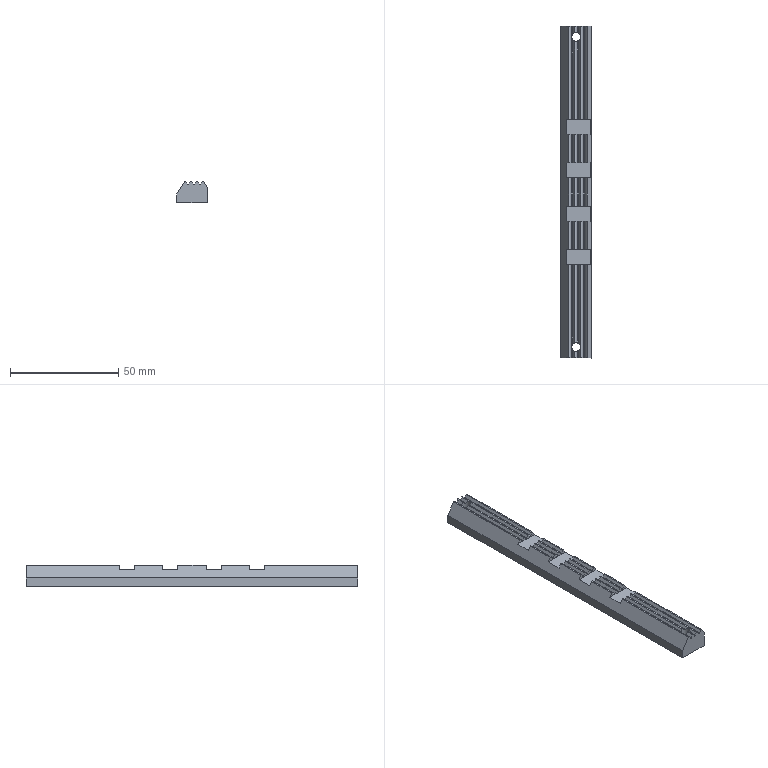Part | STEP file | 1 solid | 94 faces | box 14 x 153 x 10 mm | volume 17762 mm3 | plane 53 | cylinder 41 | commonest cylinder face diameters 0.6 x22 0.8 x17 4 x2